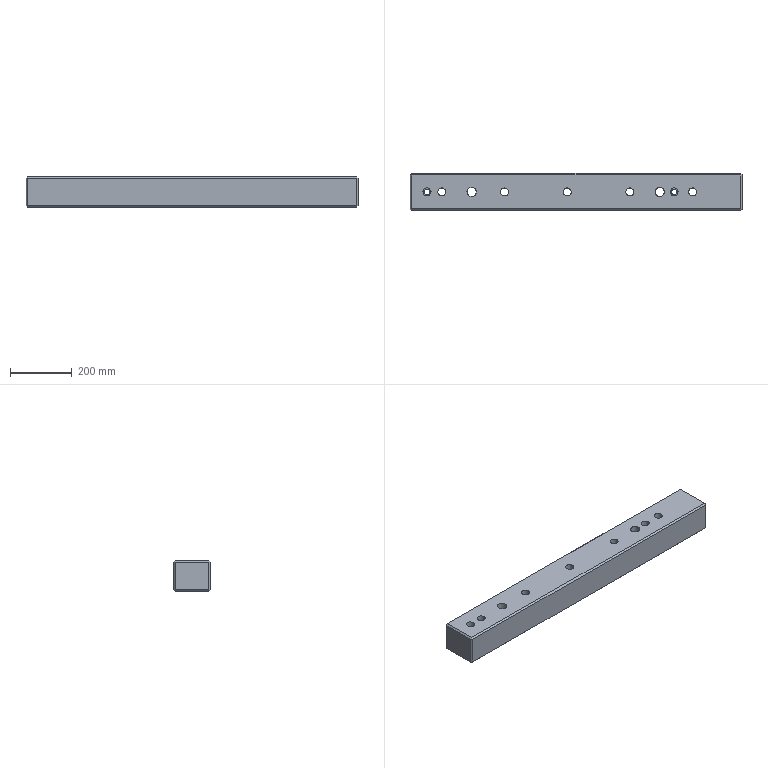Part | STEP file | solid 107 | 1 solid | 39 faces | box 1075 x 120 x 100 mm | volume 12371190 mm3 | plane 22 | cylinder 11 | spline 4 | other 2 | commonest cylinder face diameters 26 x7 17.5 x2 30 x2